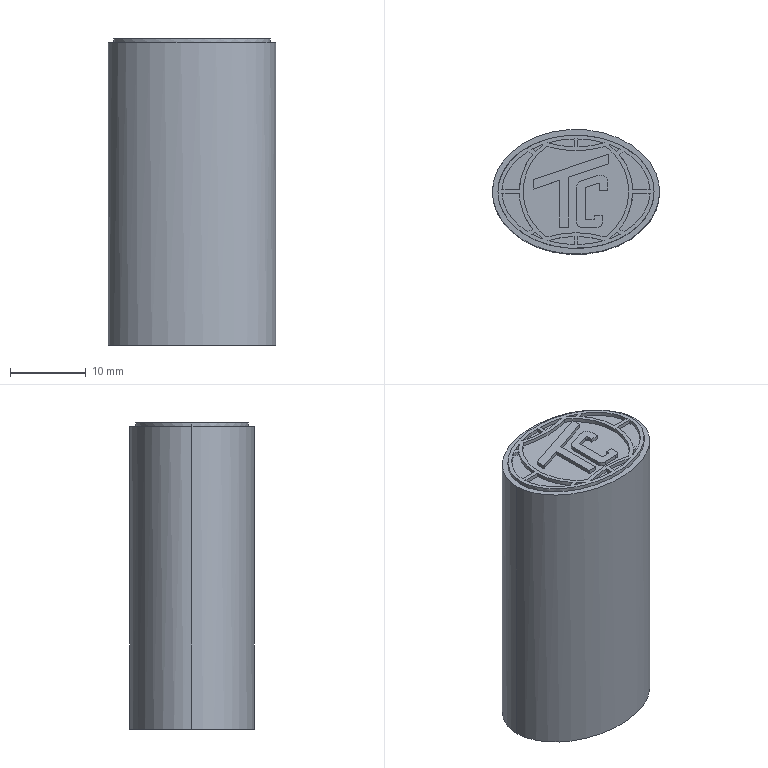Part | STEP file | LOGO LOI | 1 solid | 102 faces | box 22 x 16.4 x 40.3 mm | volume 10596 mm3 | plane 46 | spline 26 | cylinder 26 | cone 4 | commonest cylinder face diameters 26.92 x6 25.92 x4 29.02 x4 30.02 x4 0.4 x2 1.36 x2